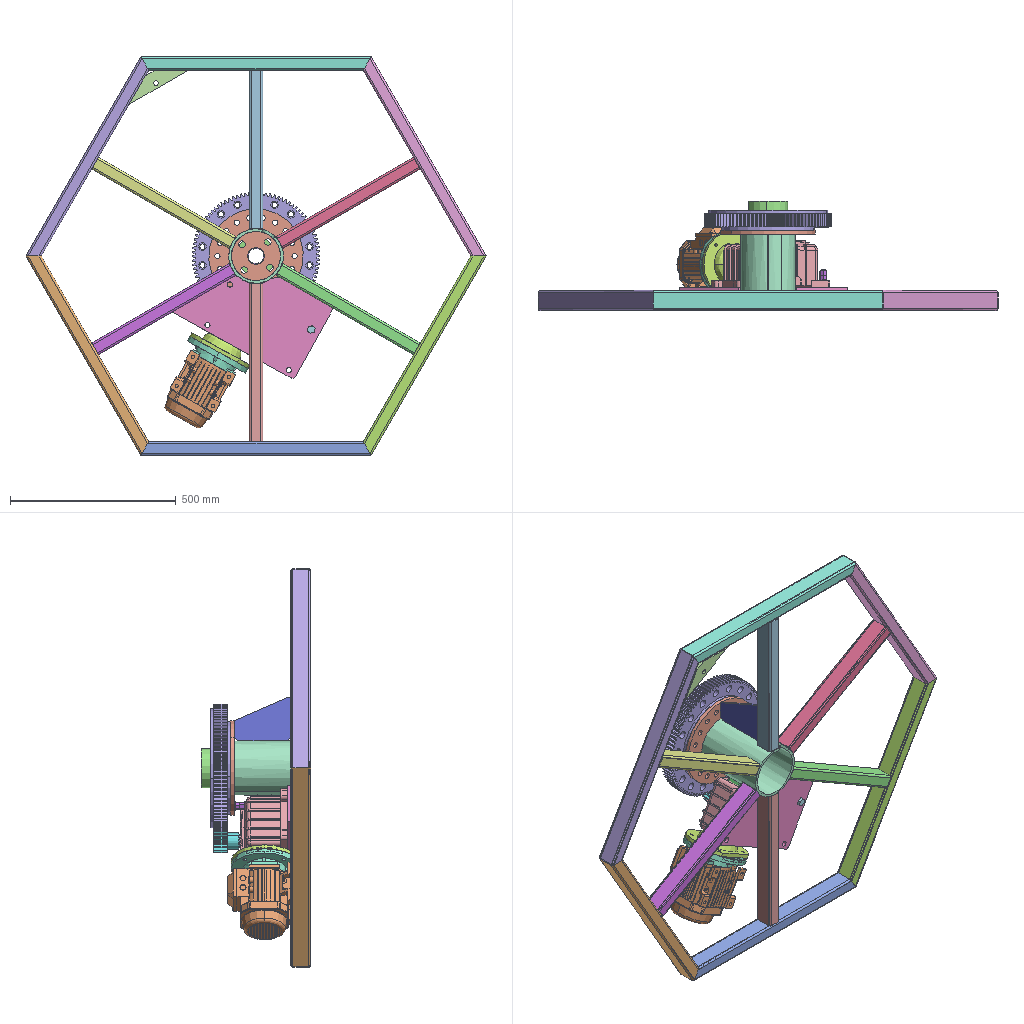Assembly | SolidWorks | 17 different items | 21 placed | box 1386 x 330 x 1200 mm
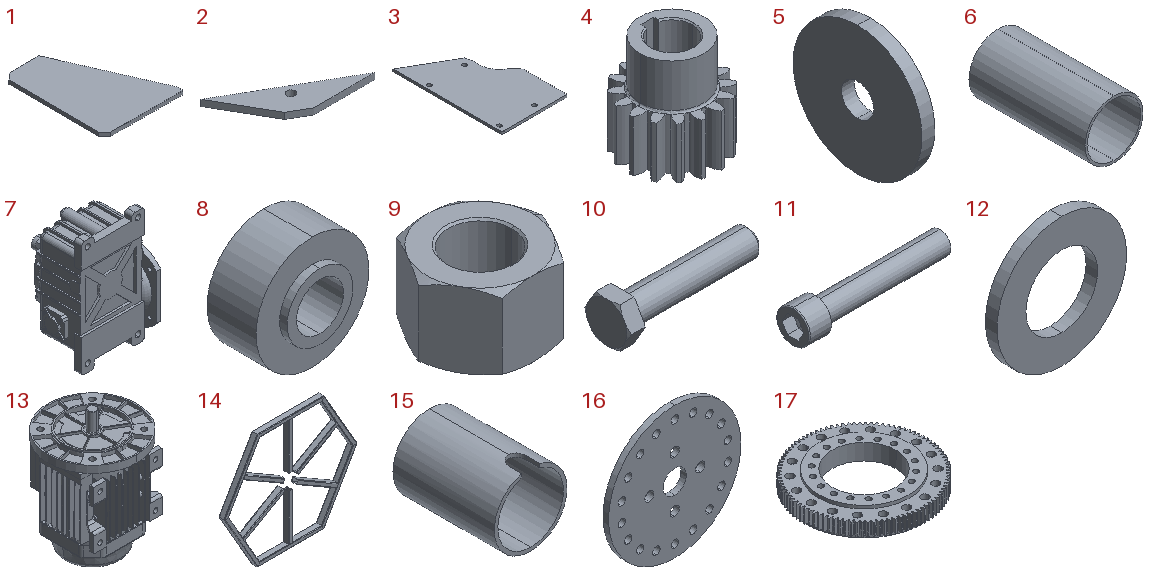Parts list (item | quantity | size | volume | features):
1 | x1 | 130 x 170 x 6 mm | 98400 mm3 | features Chamfer 1, Extrusion 1
2 | x1 | 180 x 104 x 10 mm | 59102 mm3 | features Extrusion 1
3 | x1 | 260 x 436 x 10 mm | 861786 mm3 | features Extrusion 1, Fillet 1, HoleWzd 1
4 | x1 | 71.792 x 71.792 x 75 mm | 126582 mm3 | features ICE 4, Chamfer 1, CirPattern 1, Extrusion 1, Fillet 1
5 | x1 | 4 x 40 x 40 mm | 4712 mm3 | features Extrusion 1
6 | x1 | 50 x 100 x 50 mm | 30159 mm3 | features Extrusion 1, ICE 1
7 | x1 | 226 x 220 x 326.9 mm | 6279798 mm3 | features ICE 30, DeleteBody 8, CirPattern 5, Fillet 5, MirrorSolid 4, LPattern 3, Revolution 3, Chamfer 2, Extrusion 1, MirrorPattern 1, RevCut 1
8 | x1 | 120 x 60 x 120 mm | 501084 mm3 | features Revolution 1
9 | x4 | 22.8 x 19.745 x 13.9 mm | 3143 mm3 | features Cut 2, Chamfer 1, Extrusion 1
10 | x1 | 73.8 x 24.249 x 21 mm | 13256 mm3 | features RevCut 4, Revolution 2, Chamfer 1, Extrusion 1, LPattern 1
11 | x1 | 94 x 21 x 21 mm | 16190 mm3 | features BlendCut 1, Cut 1, Fillet 1, LPattern 1, RevCut 1, Revolution 1
12 | x2 | 28 x 2.5 x 28 mm | 1068 mm3 | features Revolution 1
13 | x1 | 200 x 210 x 270 mm | 3858118 mm3 | features ICE 42, Fillet 16, MirrorPattern 8, CirPattern 7, Extrusion 5, Revolution 4, Dome 2, LPattern 2, LibraryFeature 2, Chamfer 1, CombineBodies 1, RevCut 1, Shell 1
14 | x1 | 1386 x 60 x 1200 mm | 3722678 mm3 | features WeldCornerFeat 6, CirPattern 1, RefAxis 1, WeldMemberFeat 1, WeldmentFeature 1
15 | x1 | 165 x 230 x 165 mm | 892768 mm3 | features Extrusion 1, ICE 1
16 | x1 | 285 x 12 x 285 mm | 683457 mm3 | features HoleWzd 2, Extrusion 1
17 | x1 | 383.896 x 384 x 60 mm | 3397645 mm3 | features ICE 4, HoleWzd 2, CirPattern 1, Extrusion 1
Mates (type | each side: item.copy, entity, surface, feature):
Concentric | 15.1 face cylinder Boss-Extrude1 | assembly axis
Coincident | 15.1 face plane Boss-Extrude1 | 16.1 face plane Boss-Extrude1
Concentric | 15.1 face cylinder Boss-Extrude1 | 16.1 face cylinder Boss-Extrude1
Coincident | 14.1 face plane GB/T 6728-2002 Rectangular Hollow Section 60X40X3(1) | 2.1 face plane Boss-Extrude1 | 3 times
Coincident | 14.1 face plane CirPattern1 | 1.1 face plane Boss-Extrude1
Coincident | 14.1 face plane CirPattern1 | 15.1 face plane Boss-Extrude1
PlanarAngleDim | 15.1 plane | assembly plane
Coincident | 1.1 plane | assembly plane
Tangent | 15.1 face cylinder Boss-Extrude1 | 1.1 face plane Boss-Extrude1
PlanarAngleDim | 16.1 plane | assembly plane
Concentric | 15.1 face cylinder Boss-Extrude1 | 3.1 face cylinder Boss-Extrude1
Coincident | 14.1 face plane CirPattern1 | 3.1 face plane Boss-Extrude1
Concentric | 6.1 face cylinder Boss-Extrude1 | 16.1 face cylinder Boss-Extrude1
Coincident | 16.1 face plane Boss-Extrude1 | 6.1 face plane Boss-Extrude1
Coincident | 3.1 face plane Boss-Extrude1 | 7.1 face plane Boss-Extrude2
Concentric | 3.1 face cylinder Ø16.0 (16) Diameter Hole1 | 7.1 face cylinder Boss-Extrude2 | 2 times
Concentric | 17.1 face cylinder Cut-Extrude3 | 16.1 face cylinder Boss-Extrude1
Coincident | 16.1 face plane Boss-Extrude1 | 17.1 face plane Boss-Extrude1
Concentric | 16.1 face cylinder Ø16.0 (16) Diameter Hole1 | 17.1 face cylinder Hole2
Concentric | 4.1 face cylinder Boss-Extrude1 | 7.1 face cylinder Revolve1
Coincident | 4.1 face plane Boss-Extrude1 | 17.1 face plane Cut-Extrude2
Concentric | 4.1 face cylinder Cut-Extrude1 | 5.1 face cylinder Boss-Extrude1
Coincident | 4.1 face plane Cut-Extrude1 | 5.1 face plane Boss-Extrude1
Concentric | 6.1 face cylinder Boss-Extrude1 | 8.1 face cylinder Revolve1
Coincident | 6.1 face plane Boss-Extrude1 | 8.1 face plane Revolve1
Concentric | 7.1 face cylinder Boss-Extrude2 | 10.1 face cylinder Boss-Revolve1
Coincident | 3.1 face plane Boss-Extrude1 | 10.1 face plane Boss-Extrude
Concentric | 12.1 face cylinder Boss-Revolve | 9.1 face cylinder Boss-Extrude
Concentric | 9.1 face cylinder Boss-Extrude | 9.2 face cylinder Boss-Extrude
Coincident | 12.1 face plane Boss-Revolve | 9.2 face plane Boss-Extrude
Coincident | 9.1 face plane Boss-Extrude | 9.2 face plane Boss-Extrude
Concentric | 10.1 face cylinder Boss-Revolve1 | 9.1 face cylinder Boss-Extrude
Coincident | 7.1 face plane Boss-Extrude2 | 12.1 face plane Boss-Revolve
Concentric | 17.1 face cylinder Hole2 | 11.1 face cylinder Boss-Revolve
Coincident | 17.1 face plane Hole2 | 11.1 face plane Boss-Revolve
Coincident | 12.2 face plane Boss-Revolve | 9.3 face plane Boss-Extrude
Concentric | 12.2 face cylinder Boss-Revolve | 9.4 face cylinder Boss-Extrude
Concentric | 9.3 face cylinder Boss-Extrude | 9.4 face cylinder Boss-Extrude
Coincident | 9.3 face plane Boss-Extrude | 9.4 face plane Boss-Extrude
Concentric | 11.1 face cylinder Boss-Revolve | 9.3 face cylinder Boss-Extrude
Coincident | 16.1 face plane Boss-Extrude1 | 12.2 face plane Boss-Revolve
Concentric | 7.1 face cylinder Revolve3 | 13.1 face cylinder Revolve4
Coincident | 7.1 face plane Revolve3 | 13.1 face plane Revolve4
Concentric | 7.1 face cylinder Cut-Extrude7 | 13.1 face cylinder Cut-Extrude11
DistanceDim | 4.1 face cylinder Boss-Extrude3 | 14.1 face plane GB/T 6728-2002 Rectangular Hollow Section 60X40X3(1)